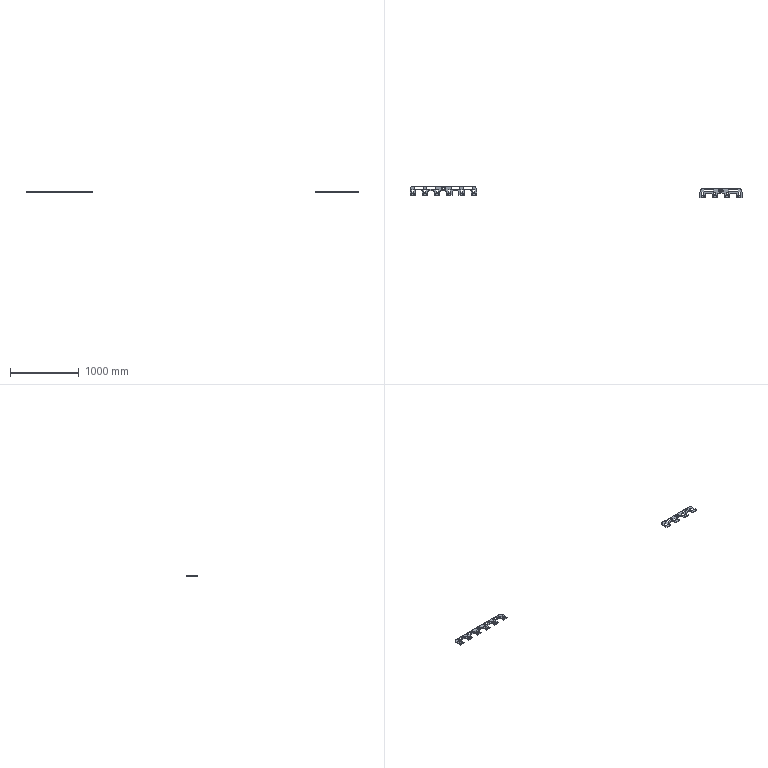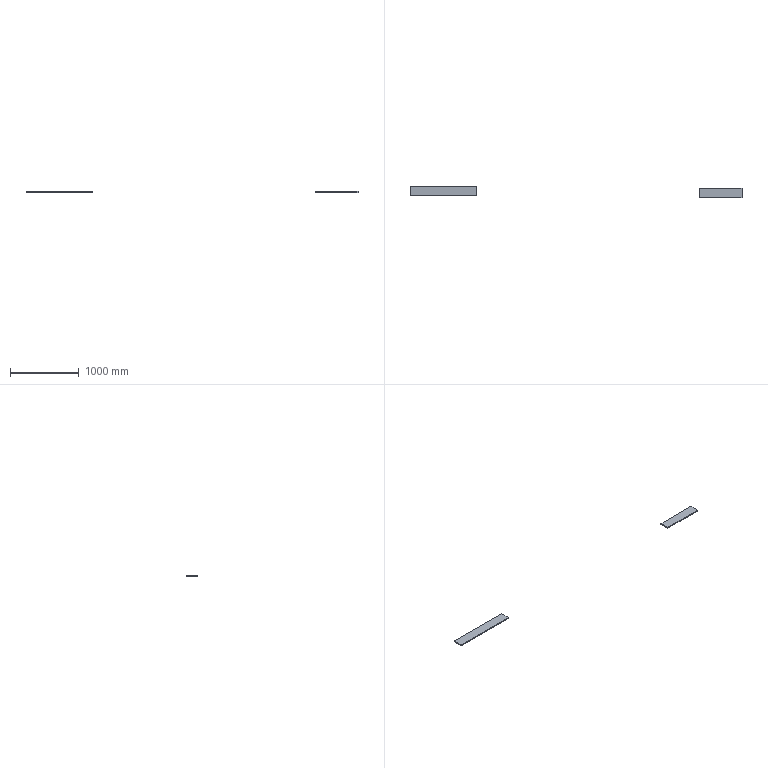CAM job | NX | 3-axis milling, drilling | part box 4825 x 168.213 x 13 mm | stock box 4829 x 172.213 x 15 mm
Tools:
number,name,description,diameter,corner_radius,flute_length,length,flutes
1,D63,Milling Tool-5 Parameters,63.0,0.0,50.0,75.0,2
7,D6A45,Milling Tool-5 Parameters,6.0,0.0,50.0,75.0,2
14,4.5ZT,Drilling Tool,4.5,0.0,35.0,50.0,2
15,6.5ZT,Drilling Tool,6.5,0.0,35.0,50.0,2
10,D10,Milling Tool-5 Parameters,10.0,0.0,50.0,75.0,2
6,D6,Milling Tool-5 Parameters,6.0,0.0,50.0,75.0,2
Operations:
program,operation,operation_type,tool,method,geometry_group,spindle_rpm,surface_speed,feed_per_tooth,feed_cut,feed_plunge,cut_length_mm,path_length_mm,cut_time_min,machine_time_min
1,FLOOR_WALL,VolumeBased25DMillingOperation,D63,METHOD,A,6500.0,1286.0,0.1154,1500.0,100.0,7031.591,7831.027,4.688,4.768
1,DRILLING,Operation,D6A45,METHOD,A,5000.0,94.0,0.025,250.0,0.0,100.0,1280.776,0.4,0.5181
1,DRILLING_COPY,Operation,4.5ZT,METHOD,A,2000.0,28.0,0.0625,250.0,0.0,146.815,526.106,0.5873,0.6252
1,DRILLING_COPY_COPY,Operation,6.5ZT,METHOD,A,2000.0,28.0,0.0625,250.0,0.0,303.245,1463.066,1.213,1.329
1,ZLEVEL_PROFILE,ZLevelMilling,D10,METHOD,A,9500.0,298.0,0.1842,3500.0,1000.0,23819.285,23888.685,6.839,6.846
1,ZLEVEL_PROFILE_COPY_2,ZLevelMilling,D10,METHOD,A,9500.0,298.0,0.1842,3500.0,1000.0,13948.182,15980.532,4.223,4.426
1,ZLEVEL_PROFILE_COPY,ZLevelMilling,D10,METHOD,A,9500.0,298.0,0.0789,1500.0,1000.0,1589.36,3617.893,1.246,1.449
1,FLOOR_WALL_1,VolumeBased25DMillingOperation,D10,METHOD,A,9500.0,298.0,0.1579,3000.0,1000.0,8605.789,9519.764,2.898,2.99
1,FLOOR_WALL_1_COPY,VolumeBased25DMillingOperation,D10,METHOD,A,9500.0,298.0,0.0789,1500.0,1000.0,2540.743,3493.669,1.701,1.796
1,HOLE_MILLING,CylinderMilling,D6,METHOD,A,9500.0,179.0,0.0737,1400.0,100.0,589.727,1252.539,0.4212,0.4875
1,ZLEVEL_PROFILE_COPY_1,ZLevelMilling,D6,METHOD,A,9500.0,179.0,0.0868,1650.0,1000.0,3669.511,8122.015,2.486,2.931
1,PLANAR_MILL,PlanarMilling,D6A45,METHOD,A,9500.0,179.0,0.0737,1400.0,100.0,2973.424,4752.001,2.124,2.302
1,PLANAR_MILL_COPY,PlanarMilling,D6A45,METHOD,A,9500.0,179.0,0.0737,1400.0,100.0,901.954,4016.834,0.6443,0.9557
1,ZLEVEL_PROFILE_COPY_COPY,ZLevelMilling,D10,METHOD,A,9500.0,298.0,0.0632,1200.0,1000.0,7309.408,7392.708,6.092,6.101
1111,FLOOR_WALL_COPY,VolumeBased25DMillingOperation,D63,METHOD,B,6500.0,1286.0,0.1154,1500.0,100.0,10587.592,11739.492,7.058,7.174
1111,DRILLING_COPY_1,Operation,D6A45,METHOD,B,5000.0,94.0,0.025,250.0,0.0,132.0,1815.225,0.528,0.6963
1111,DRILLING_COPY_COPY_1,Operation,4.5ZT,METHOD,B,2000.0,28.0,0.0625,250.0,0.0,146.815,526.106,0.5873,0.6252
1111,DRILLING_COPY_COPY_COPY,Operation,6.5ZT,METHOD,B,2000.0,28.0,0.0625,250.0,0.0,454.867,2236.76,1.819,1.998
1111,ZLEVEL_PROFILE_COPY_3,ZLevelMilling,D10,METHOD,B,9500.0,298.0,0.1842,3500.0,1000.0,36884.606,36954.006,10.573,10.579
1111,ZLEVEL_PROFILE_COPY_2_COPY,ZLevelMilling,D10,METHOD,B,9500.0,298.0,0.1842,3500.0,1000.0,25934.527,29042.423,7.785,8.096
1111,ZLEVEL_PROFILE_COPY_COPY_1,ZLevelMilling,D10,METHOD,B,9500.0,298.0,0.0789,1500.0,1000.0,6947.395,9493.318,4.716,4.971
1111,FLOOR_WALL_1_COPY_1,VolumeBased25DMillingOperation,D10,METHOD,B,9500.0,298.0,0.1579,3000.0,1000.0,12908.684,14367.827,4.347,4.493
1111,FLOOR_WALL_1_COPY_COPY,VolumeBased25DMillingOperation,D10,METHOD,B,9500.0,298.0,0.0789,1500.0,1000.0,3811.115,5280.913,2.551,2.698
1111,HOLE_MILLING_COPY,CylinderMilling,D6,METHOD,B,9500.0,179.0,0.0737,1400.0,100.0,589.727,1252.539,0.4212,0.4875
1111,ZLEVEL_PROFILE_COPY_1_COPY,ZLevelMilling,D6,METHOD,B,9500.0,179.0,0.0868,1650.0,1000.0,6116.234,14253.739,4.144,4.957
1111,PLANAR_MILL_COPY_1,PlanarMilling,D6A45,METHOD,B,9500.0,179.0,0.0737,1400.0,100.0,4768.729,7248.01,3.406,3.654
1111,PLANAR_MILL_COPY_COPY,PlanarMilling,D6A45,METHOD,B,9500.0,179.0,0.0737,1400.0,100.0,1352.931,5827.391,0.9664,1.414
1111,ZLEVEL_PROFILE_COPY_3_COPY,ZLevelMilling,D10,METHOD,B,9500.0,298.0,0.0632,1200.0,1000.0,11340.341,11415.766,9.452,9.459
2222,FLOOR_WALL_COPY_COPY,VolumeBased25DMillingOperation,D63,METHOD,C,6500.0,1286.0,0.1154,1500.0,100.0,5215.19,5462.186,3.477,3.502
2222,DRILLING_COPY_1_COPY,Operation,D6A45,METHOD,C,5000.0,94.0,0.025,250.0,0.0,32.0,451.872,0.128,0.17
2222,DRILLING_COPY_COPY_COPY_COPY,Operation,6.5ZT,METHOD,C,2000.0,28.0,0.0625,250.0,0.0,151.622,691.116,0.6065,0.6604
2222,ZLEVEL_PROFILE_COPY_3_COPY_1,ZLevelMilling,D10,METHOD,C,9500.0,298.0,0.1842,3500.0,1000.0,15087.127,15909.727,4.399,4.481
2222,ZLEVEL_PROFILE_COPY_2_COPY_COPY,ZLevelMilling,D10,METHOD,C,9500.0,298.0,0.1842,3500.0,1000.0,10992.944,11842.594,3.277,3.362
2222,ZLEVEL_PROFILE_COPY_COPY_1_COPY,ZLevelMilling,D10,METHOD,C,9500.0,298.0,0.0789,1500.0,1000.0,2944.108,3775.286,1.994,2.077
2222,FLOOR_WALL_1_COPY_1_COPY,VolumeBased25DMillingOperation,D10,METHOD,C,9500.0,298.0,0.1579,3000.0,1000.0,4302.895,4676.298,1.449,1.486
2222,FLOOR_WALL_1_COPY_COPY_COPY,VolumeBased25DMillingOperation,D10,METHOD,C,9500.0,298.0,0.0789,1500.0,1000.0,1270.372,1653.688,0.8503,0.8886
2222,ZLEVEL_PROFILE_COPY_1_COPY_COPY,ZLevelMilling,D6,METHOD,C,9500.0,179.0,0.0868,1650.0,1000.0,2446.574,5208.05,1.657,1.934
2222,PLANAR_MILL_COPY_1_COPY,PlanarMilling,D6A45,METHOD,C,9500.0,179.0,0.0737,1400.0,100.0,1978.318,3132.882,1.413,1.528
2222,PLANAR_MILL_COPY_COPY_COPY,PlanarMilling,D6A45,METHOD,C,9500.0,179.0,0.0737,1400.0,100.0,450.977,1752.168,0.3221,0.4522
2222,ZLEVEL_PROFILE_COPY_3_COPY_COPY,ZLevelMilling,D10,METHOD,C,9500.0,298.0,0.0632,1200.0,1000.0,4640.936,5395.636,3.874,3.949